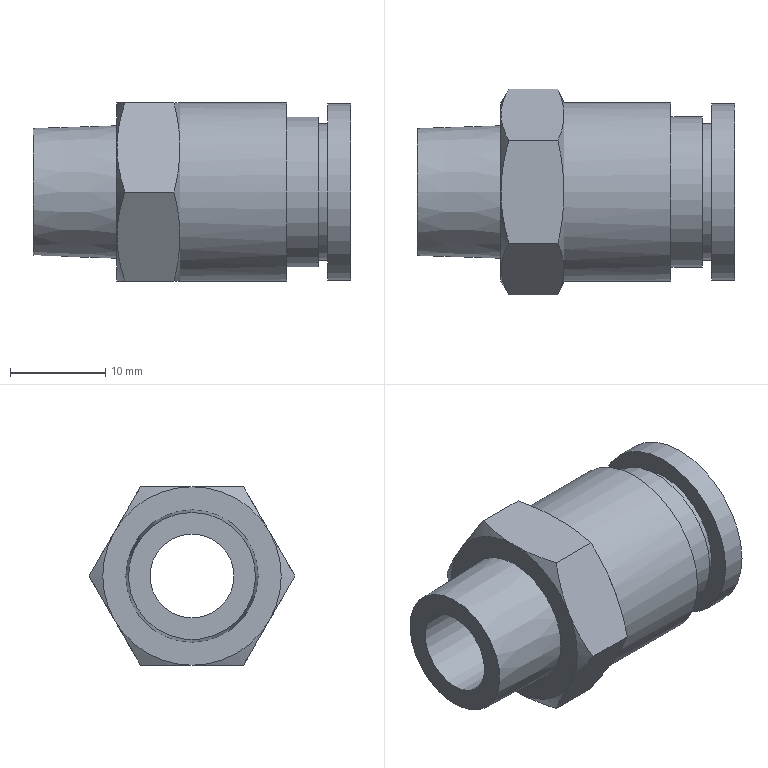Part | NX | features 模具.stp<1>[85] 2 | 1 solid | 32 faces | box 33.33 x 21.593 x 18.7 mm | volume 4989 mm3 | plane 13 | cone 13 | cylinder 6 | commonest cylinder face diameters 8.8 x1 11 x1 14.3 x1 15.73 x1 18.48 x1 18.7 x1
STEP:
#1=CARTESIAN_POINT('',(281.76,-25.,-59.9));
#2=VERTEX_POINT('',#1);
#3=CARTESIAN_POINT('',(281.76,-25.,-55.5));
#4=DIRECTION('',(-1.,0.,0.));
#5=DIRECTION('',(0.,0.,-1.));
#6=AXIS2_PLACEMENT_3D('',#3,#4,#5);
#7=CIRCLE('',#6,4.4);
#8=EDGE_CURVE('',#2,#2,#7,.T.);
#9=ORIENTED_EDGE('',*,*,#8,.F.);
#10=EDGE_LOOP('',(#9));
#11=FACE_BOUND('',#10,.T.);
#12=CARTESIAN_POINT('',(271.2,-25.,-51.1));
#13=VERTEX_POINT('',#12);
#14=CARTESIAN_POINT('',(271.2,-25.,-55.5));
#15=DIRECTION('',(-1.,0.,0.));
#16=DIRECTION('',(0.,0.,1.));
#17=AXIS2_PLACEMENT_3D('',#14,#15,#16);
#18=CIRCLE('',#17,4.4);
#19=EDGE_CURVE('',#13,#13,#18,.T.);
#20=ORIENTED_EDGE('',*,*,#19,.T.);
#21=EDGE_LOOP('',(#20));
#22=FACE_BOUND('',#21,.T.);
#23=CARTESIAN_POINT('',(304.53,-25.,-55.5));
#24=DIRECTION('',(1.,0.,0.));
#25=DIRECTION('',(0.,0.,1.));
#26=AXIS2_PLACEMENT_3D('',#23,#24,#25);
#27=CYLINDRICAL_SURFACE('',#26,4.4);
#28=ADVANCED_FACE('',(#11,#22),#27,.F.);
#29=ORIENTED_EDGE('',*,*,#8,.T.);
#30=EDGE_LOOP('',(#29));
#31=FACE_BOUND('',#30,.T.);
#32=CARTESIAN_POINT('',(281.76,-25.,-50.));
#33=VERTEX_POINT('',#32);
#34=CARTESIAN_POINT('',(281.76,-25.,-55.5));
#35=DIRECTION('',(-1.,0.,0.));
#36=DIRECTION('',(0.,0.,1.));
#37=AXIS2_PLACEMENT_3D('',#34,#35,#36);
#38=CIRCLE('',#37,5.5);
#39=EDGE_CURVE('',#33,#33,#38,.T.);
#40=ORIENTED_EDGE('',*,*,#39,.F.);
#41=EDGE_LOOP('',(#40));
#42=FACE_BOUND('',#41,.T.);
#43=CARTESIAN_POINT('',(281.76,-18.4,-48.9));
#44=DIRECTION('',(-1.,0.,0.));
#45=DIRECTION('',(0.,0.,1.));
#46=AXIS2_PLACEMENT_3D('',#43,#44,#45);
#47=PLANE('',#46);
#48=ADVANCED_FACE('',(#31,#42),#47,.F.);
#49=CARTESIAN_POINT('',(304.53,-25.,-61.));
#50=VERTEX_POINT('',#49);
#51=CARTESIAN_POINT('',(304.53,-25.,-55.5));
#52=DIRECTION('',(-1.,0.,0.));
#53=DIRECTION('',(0.,0.,-1.));
#54=AXIS2_PLACEMENT_3D('',#51,#52,#53);
#55=CIRCLE('',#54,5.5);
#56=EDGE_CURVE('',#50,#50,#55,.T.);
#57=ORIENTED_EDGE('',*,*,#56,.F.);
#58=EDGE_LOOP('',(#57));
#59=FACE_BOUND('',#58,.T.);
#60=ORIENTED_EDGE('',*,*,#39,.T.);
#61=EDGE_LOOP('',(#60));
#62=FACE_BOUND('',#61,.T.);
#63=CARTESIAN_POINT('',(304.53,-25.,-55.5));
#64=DIRECTION('',(1.,0.,0.));
#65=DIRECTION('',(0.,0.,1.));
#66=AXIS2_PLACEMENT_3D('',#63,#64,#65);
#67=CYLINDRICAL_SURFACE('',#66,5.5);
#68=ADVANCED_FACE('',(#59,#62),#67,.F.);
#69=ORIENTED_EDGE('',*,*,#56,.T.);
#70=EDGE_LOOP('',(#69));
#71=FACE_BOUND('',#70,.T.);
#72=CARTESIAN_POINT('',(304.53,-34.24,-55.5));
#73=VERTEX_POINT('',#72);
#74=CARTESIAN_POINT('',(304.53,-25.,-55.5));
#75=DIRECTION('',(1.,0.,0.));
#76=DIRECTION('',(0.,-1.,0.));
#77=AXIS2_PLACEMENT_3D('',#74,#75,#76);
#78=CIRCLE('',#77,9.24);
#79=EDGE_CURVE('',#73,#73,#78,.T.);
#80=ORIENTED_EDGE('',*,*,#79,.T.);
#81=EDGE_LOOP('',(#80));
#82=FACE_BOUND('',#81,.T.);
#83=CARTESIAN_POINT('',(304.53,-36.088,-66.588));
#84=DIRECTION('',(1.,0.,0.));
#85=DIRECTION('',(0.,1.,0.));
#86=AXIS2_PLACEMENT_3D('',#83,#84,#85);
#87=PLANE('',#86);
#88=ADVANCED_FACE('',(#71,#82),#87,.T.);
#89=CARTESIAN_POINT('',(302.11,-15.76,-55.5));
#90=VERTEX_POINT('',#89);
#91=CARTESIAN_POINT('',(302.11,-25.,-55.5));
#92=DIRECTION('',(1.,0.,0.));
#93=DIRECTION('',(0.,1.,0.));
#94=AXIS2_PLACEMENT_3D('',#91,#92,#93);
#95=CIRCLE('',#94,9.24);
#96=EDGE_CURVE('',#90,#90,#95,.T.);
#97=ORIENTED_EDGE('',*,*,#96,.T.);
#98=EDGE_LOOP('',(#97));
#99=FACE_BOUND('',#98,.T.);
#100=ORIENTED_EDGE('',*,*,#79,.F.);
#101=EDGE_LOOP('',(#100));
#102=FACE_BOUND('',#101,.T.);
#103=CARTESIAN_POINT('',(302.11,-25.,-55.5));
#104=DIRECTION('',(-1.,0.,0.));
#105=DIRECTION('',(0.,-1.,0.));
#106=AXIS2_PLACEMENT_3D('',#103,#104,#105);
#107=CYLINDRICAL_SURFACE('',#106,9.24);
#108=ADVANCED_FACE('',(#99,#102),#107,.T.);
#109=CARTESIAN_POINT('',(302.11,-32.15,-55.5));
#110=VERTEX_POINT('',#109);
#111=CARTESIAN_POINT('',(302.11,-25.,-55.5));
#112=DIRECTION('',(1.,0.,0.));
#113=DIRECTION('',(0.,-1.,0.));
#114=AXIS2_PLACEMENT_3D('',#111,#112,#113);
#115=CIRCLE('',#114,7.15);
#116=EDGE_CURVE('',#110,#110,#115,.T.);
#117=ORIENTED_EDGE('',*,*,#116,.T.);
#118=EDGE_LOOP('',(#117));
#119=FACE_BOUND('',#118,.T.);
#120=ORIENTED_EDGE('',*,*,#96,.F.);
#121=EDGE_LOOP('',(#120));
#122=FACE_BOUND('',#121,.T.);
#123=CARTESIAN_POINT('',(302.11,-36.088,-66.588));
#124=DIRECTION('',(1.,0.,0.));
#125=DIRECTION('',(0.,1.,0.));
#126=AXIS2_PLACEMENT_3D('',#123,#124,#125);
#127=PLANE('',#126);
#128=ADVANCED_FACE('',(#119,#122),#127,.F.);
#129=CARTESIAN_POINT('',(301.12,-17.85,-55.5));
#130=VERTEX_POINT('',#129);
#131=CARTESIAN_POINT('',(301.12,-25.,-55.5));
#132=DIRECTION('',(1.,0.,0.));
#133=DIRECTION('',(0.,1.,0.));
#134=AXIS2_PLACEMENT_3D('',#131,#132,#133);
#135=CIRCLE('',#134,7.15);
#136=EDGE_CURVE('',#130,#130,#135,.T.);
#137=ORIENTED_EDGE('',*,*,#136,.T.);
#138=EDGE_LOOP('',(#137));
#139=FACE_BOUND('',#138,.T.);
#140=ORIENTED_EDGE('',*,*,#116,.F.);
#141=EDGE_LOOP('',(#140));
#142=FACE_BOUND('',#141,.T.);
#143=CARTESIAN_POINT('',(301.12,-25.,-55.5));
#144=DIRECTION('',(-1.,0.,0.));
#145=DIRECTION('',(0.,-1.,0.));
#146=AXIS2_PLACEMENT_3D('',#143,#144,#145);
#147=CYLINDRICAL_SURFACE('',#146,7.15);
#148=ADVANCED_FACE('',(#139,#142),#147,.T.);
#149=ORIENTED_EDGE('',*,*,#136,.F.);
#150=EDGE_LOOP('',(#149));
#151=FACE_BOUND('',#150,.T.);
#152=CARTESIAN_POINT('',(301.12,-32.865,-55.5));
#153=VERTEX_POINT('',#152);
#154=CARTESIAN_POINT('',(301.12,-25.,-55.5));
#155=DIRECTION('',(1.,0.,0.));
#156=DIRECTION('',(0.,-1.,0.));
#157=AXIS2_PLACEMENT_3D('',#154,#155,#156);
#158=CIRCLE('',#157,7.865);
#159=EDGE_CURVE('',#153,#153,#158,.T.);
#160=ORIENTED_EDGE('',*,*,#159,.T.);
#161=EDGE_LOOP('',(#160));
#162=FACE_BOUND('',#161,.T.);
#163=CARTESIAN_POINT('',(301.12,-34.438,-64.938));
#164=DIRECTION('',(1.,0.,0.));
#165=DIRECTION('',(0.,1.,0.));
#166=AXIS2_PLACEMENT_3D('',#163,#164,#165);
#167=PLANE('',#166);
#168=ADVANCED_FACE('',(#151,#162),#167,.T.);
#169=CARTESIAN_POINT('',(297.82,-17.135,-55.5));
#170=VERTEX_POINT('',#169);
#171=CARTESIAN_POINT('',(297.82,-25.,-55.5));
#172=DIRECTION('',(1.,0.,0.));
#173=DIRECTION('',(0.,1.,0.));
#174=AXIS2_PLACEMENT_3D('',#171,#172,#173);
#175=CIRCLE('',#174,7.865);
#176=EDGE_CURVE('',#170,#170,#175,.T.);
#177=ORIENTED_EDGE('',*,*,#176,.T.);
#178=EDGE_LOOP('',(#177));
#179=FACE_BOUND('',#178,.T.);
#180=ORIENTED_EDGE('',*,*,#159,.F.);
#181=EDGE_LOOP('',(#180));
#182=FACE_BOUND('',#181,.T.);
#183=CARTESIAN_POINT('',(297.82,-25.,-55.5));
#184=DIRECTION('',(-1.,0.,0.));
#185=DIRECTION('',(0.,-1.,0.));
#186=AXIS2_PLACEMENT_3D('',#183,#184,#185);
#187=CYLINDRICAL_SURFACE('',#186,7.865);
#188=ADVANCED_FACE('',(#179,#182),#187,.T.);
#189=ORIENTED_EDGE('',*,*,#176,.F.);
#190=EDGE_LOOP('',(#189));
#191=FACE_BOUND('',#190,.T.);
#192=CARTESIAN_POINT('',(297.82,-15.65,-55.5));
#193=VERTEX_POINT('',#192);
#194=CARTESIAN_POINT('',(297.82,-25.,-55.5));
#195=DIRECTION('',(1.,0.,0.));
#196=DIRECTION('',(0.,1.,0.));
#197=AXIS2_PLACEMENT_3D('',#194,#195,#196);
#198=CIRCLE('',#197,9.35);
#199=EDGE_CURVE('',#193,#193,#198,.T.);
#200=ORIENTED_EDGE('',*,*,#199,.T.);
#201=EDGE_LOOP('',(#200));
#202=FACE_BOUND('',#201,.T.);
#203=CARTESIAN_POINT('',(297.82,-36.22,-66.72));
#204=DIRECTION('',(1.,0.,0.));
#205=DIRECTION('',(0.,1.,0.));
#206=AXIS2_PLACEMENT_3D('',#203,#204,#205);
#207=PLANE('',#206);
#208=ADVANCED_FACE('',(#191,#202),#207,.T.);
#209=CARTESIAN_POINT('',(285.975,-19.602,-46.15));
#210=VERTEX_POINT('',#209);
#211=CARTESIAN_POINT('',(286.6,-25.,-46.15));
#212=VERTEX_POINT('',#211);
#213=CARTESIAN_POINT('',(286.6,-25.,-46.15));
#214=CARTESIAN_POINT('',(286.6,-24.126,-46.15));
#215=CARTESIAN_POINT('',(286.487,-22.321,-46.15));
#216=CARTESIAN_POINT('',(286.183,-20.564,-46.15));
#217=CARTESIAN_POINT('',(285.975,-19.602,-46.15));
#218=B_SPLINE_CURVE_WITH_KNOTS('',3,(#213,#214,#215,#216,#217),.UNSPECIFIED.,.F.,.F.,(4,1,4),(0.,0.5,1.),.UNSPECIFIED.);
#219=EDGE_CURVE('',#210,#212,#218,.F.);
#220=ORIENTED_EDGE('',*,*,#219,.F.);
#221=CARTESIAN_POINT('',(280.835,-19.602,-46.15));
#222=VERTEX_POINT('',#221);
#223=CARTESIAN_POINT('',(280.835,-19.602,-46.15));
#224=DIRECTION('',(1.,0.,0.));
#225=VECTOR('',#224,1000.);
#226=LINE('',#223,#225);
#227=EDGE_CURVE('',#222,#210,#226,.T.);
#228=ORIENTED_EDGE('',*,*,#227,.F.);
#229=CARTESIAN_POINT('',(280.,-25.,-46.15));
#230=VERTEX_POINT('',#229);
#231=CARTESIAN_POINT('',(280.835,-19.602,-46.15));
#232=CARTESIAN_POINT('',(280.557,-20.566,-46.15));
#233=CARTESIAN_POINT('',(280.149,-22.33,-46.15));
#234=CARTESIAN_POINT('',(280.,-24.127,-46.15));
#235=CARTESIAN_POINT('',(280.,-25.,-46.15));
#236=B_SPLINE_CURVE_WITH_KNOTS('',3,(#231,#232,#233,#234,#235),.UNSPECIFIED.,.F.,.F.,(4,1,4),(0.,0.5,1.),.UNSPECIFIED.);
#237=EDGE_CURVE('',#230,#222,#236,.F.);
#238=ORIENTED_EDGE('',*,*,#237,.F.);
#239=CARTESIAN_POINT('',(280.835,-30.398,-46.15));
#240=VERTEX_POINT('',#239);
#241=CARTESIAN_POINT('',(280.,-25.,-46.15));
#242=CARTESIAN_POINT('',(280.,-25.871,-46.15));
#243=CARTESIAN_POINT('',(280.147,-27.657,-46.15));
#244=CARTESIAN_POINT('',(280.556,-29.43,-46.15));
#245=CARTESIAN_POINT('',(280.835,-30.398,-46.15));
#246=B_SPLINE_CURVE_WITH_KNOTS('',3,(#241,#242,#243,#244,#245),.UNSPECIFIED.,.F.,.F.,(4,1,4),(0.,0.5,1.),.UNSPECIFIED.);
#247=EDGE_CURVE('',#240,#230,#246,.F.);
#248=ORIENTED_EDGE('',*,*,#247,.F.);
#249=CARTESIAN_POINT('',(285.975,-30.398,-46.15));
#250=VERTEX_POINT('',#249);
#251=CARTESIAN_POINT('',(280.835,-30.398,-46.15));
#252=DIRECTION('',(1.,0.,0.));
#253=VECTOR('',#252,1000.);
#254=LINE('',#251,#253);
#255=EDGE_CURVE('',#240,#250,#254,.T.);
#256=ORIENTED_EDGE('',*,*,#255,.T.);
#257=CARTESIAN_POINT('',(285.975,-30.398,-46.15));
#258=CARTESIAN_POINT('',(286.182,-29.439,-46.15));
#259=CARTESIAN_POINT('',(286.486,-27.691,-46.15));
#260=CARTESIAN_POINT('',(286.6,-25.876,-46.15));
#261=CARTESIAN_POINT('',(286.6,-25.,-46.15));
#262=B_SPLINE_CURVE_WITH_KNOTS('',3,(#257,#258,#259,#260,#261),.UNSPECIFIED.,.F.,.F.,(4,1,4),(0.,0.5,1.),.UNSPECIFIED.);
#263=EDGE_CURVE('',#212,#250,#262,.F.);
#264=ORIENTED_EDGE('',*,*,#263,.F.);
#265=EDGE_LOOP('',(#220,#228,#238,#248,#256,#264));
#266=FACE_BOUND('',#265,.T.);
#267=CARTESIAN_POINT('',(287.26,-18.522,-46.15));
#268=DIRECTION('',(0.,0.,1.));
#269=DIRECTION('',(1.,0.,0.));
#270=AXIS2_PLACEMENT_3D('',#267,#268,#269);
#271=PLANE('',#270);
#272=ADVANCED_FACE('',(#266),#271,.T.);
#273=ORIENTED_EDGE('',*,*,#255,.F.);
#274=CARTESIAN_POINT('',(280.,-33.097,-50.825));
#275=VERTEX_POINT('',#274);
#276=CARTESIAN_POINT('',(280.835,-30.398,-46.15));
#277=CARTESIAN_POINT('',(280.275,-31.368,-47.831));
#278=CARTESIAN_POINT('',(280.,-32.228,-49.319));
#279=CARTESIAN_POINT('',(280.,-33.097,-50.825));
#280=B_SPLINE_CURVE_WITH_KNOTS('',3,(#276,#277,#278,#279),.UNSPECIFIED.,.F.,.F.,(4,4),(0.,1.),.UNSPECIFIED.);
#281=EDGE_CURVE('',#275,#240,#280,.F.);
#282=ORIENTED_EDGE('',*,*,#281,.F.);
#283=CARTESIAN_POINT('',(280.835,-35.796,-55.5));
#284=VERTEX_POINT('',#283);
#285=CARTESIAN_POINT('',(280.,-33.097,-50.825));
#286=CARTESIAN_POINT('',(280.,-33.966,-52.33));
#287=CARTESIAN_POINT('',(280.275,-34.826,-53.819));
#288=CARTESIAN_POINT('',(280.835,-35.796,-55.5));
#289=B_SPLINE_CURVE_WITH_KNOTS('',3,(#285,#286,#287,#288),.UNSPECIFIED.,.F.,.F.,(4,4),(0.,1.),.UNSPECIFIED.);
#290=EDGE_CURVE('',#284,#275,#289,.F.);
#291=ORIENTED_EDGE('',*,*,#290,.F.);
#292=CARTESIAN_POINT('',(285.975,-35.796,-55.5));
#293=VERTEX_POINT('',#292);
#294=CARTESIAN_POINT('',(280.835,-35.796,-55.5));
#295=DIRECTION('',(1.,0.,0.));
#296=VECTOR('',#295,1000.);
#297=LINE('',#294,#296);
#298=EDGE_CURVE('',#284,#293,#297,.T.);
#299=ORIENTED_EDGE('',*,*,#298,.T.);
#300=CARTESIAN_POINT('',(286.6,-33.097,-50.825));
#301=VERTEX_POINT('',#300);
#302=CARTESIAN_POINT('',(285.975,-35.796,-55.5));
#303=CARTESIAN_POINT('',(286.183,-35.314,-54.665));
#304=CARTESIAN_POINT('',(286.489,-34.431,-53.136));
#305=CARTESIAN_POINT('',(286.6,-33.534,-51.581));
#306=CARTESIAN_POINT('',(286.6,-33.097,-50.825));
#307=B_SPLINE_CURVE_WITH_KNOTS('',3,(#302,#303,#304,#305,#306),.UNSPECIFIED.,.F.,.F.,(4,1,4),(0.,0.5,1.),.UNSPECIFIED.);
#308=EDGE_CURVE('',#301,#293,#307,.F.);
#309=ORIENTED_EDGE('',*,*,#308,.F.);
#310=CARTESIAN_POINT('',(286.6,-33.097,-50.825));
#311=CARTESIAN_POINT('',(286.6,-32.661,-50.069));
#312=CARTESIAN_POINT('',(286.489,-31.763,-48.514));
#313=CARTESIAN_POINT('',(286.184,-30.881,-46.986));
#314=CARTESIAN_POINT('',(285.975,-30.398,-46.15));
#315=B_SPLINE_CURVE_WITH_KNOTS('',3,(#310,#311,#312,#313,#314),.UNSPECIFIED.,.F.,.F.,(4,1,4),(0.,0.5,1.),.UNSPECIFIED.);
#316=EDGE_CURVE('',#250,#301,#315,.F.);
#317=ORIENTED_EDGE('',*,*,#316,.F.);
#318=EDGE_LOOP('',(#273,#282,#291,#299,#309,#317));
#319=FACE_BOUND('',#318,.T.);
#320=CARTESIAN_POINT('',(287.26,-29.858,-45.215));
#321=DIRECTION('',(0.,-0.866,0.5));
#322=DIRECTION('',(-1.,0.,0.));
#323=AXIS2_PLACEMENT_3D('',#320,#321,#322);
#324=PLANE('',#323);
#325=ADVANCED_FACE('',(#319),#324,.T.);
#326=CARTESIAN_POINT('',(280.,-25.,-55.5));
#327=DIRECTION('',(-1.,0.,0.));
#328=DIRECTION('',(0.,0.866,-0.5));
#329=AXIS2_PLACEMENT_3D('',#326,#327,#328);
#330=CIRCLE('',#329,9.35);
#331=EDGE_CURVE('',#275,#230,#330,.T.);
#332=ORIENTED_EDGE('',*,*,#331,.F.);
#333=ORIENTED_EDGE('',*,*,#281,.T.);
#334=ORIENTED_EDGE('',*,*,#247,.T.);
#335=EDGE_LOOP('',(#332,#333,#334));
#336=FACE_BOUND('',#335,.T.);
#337=CARTESIAN_POINT('',(281.744,-25.,-55.5));
#338=DIRECTION('',(1.,0.,0.));
#339=DIRECTION('',(0.,-0.8661,0.4999));
#340=AXIS2_PLACEMENT_3D('',#337,#338,#339);
#341=CONICAL_SURFACE('',#340,12.37,1.047);
#342=ADVANCED_FACE('',(#336),#341,.T.);
#343=CARTESIAN_POINT('',(280.,-33.097,-60.175));
#344=VERTEX_POINT('',#343);
#345=CARTESIAN_POINT('',(280.,-25.,-55.5));
#346=DIRECTION('',(-1.,0.,0.));
#347=DIRECTION('',(0.,0.866,0.5));
#348=AXIS2_PLACEMENT_3D('',#345,#346,#347);
#349=CIRCLE('',#348,9.35);
#350=EDGE_CURVE('',#344,#275,#349,.T.);
#351=ORIENTED_EDGE('',*,*,#350,.F.);
#352=CARTESIAN_POINT('',(280.835,-35.796,-55.5));
#353=CARTESIAN_POINT('',(280.275,-34.826,-57.181));
#354=CARTESIAN_POINT('',(280.,-33.967,-58.669));
#355=CARTESIAN_POINT('',(280.,-33.097,-60.175));
#356=B_SPLINE_CURVE_WITH_KNOTS('',3,(#352,#353,#354,#355),.UNSPECIFIED.,.F.,.F.,(4,4),(0.,1.),.UNSPECIFIED.);
#357=EDGE_CURVE('',#344,#284,#356,.F.);
#358=ORIENTED_EDGE('',*,*,#357,.T.);
#359=ORIENTED_EDGE('',*,*,#290,.T.);
#360=EDGE_LOOP('',(#351,#358,#359));
#361=FACE_BOUND('',#360,.T.);
#362=CARTESIAN_POINT('',(281.395,-25.,-55.5));
#363=DIRECTION('',(1.,0.,0.));
#364=DIRECTION('',(0.,0.,1.));
#365=AXIS2_PLACEMENT_3D('',#362,#363,#364);
#366=CONICAL_SURFACE('',#365,11.767,1.047);
#367=ADVANCED_FACE('',(#361),#366,.T.);
#368=CARTESIAN_POINT('',(280.,-25.,-64.85));
#369=VERTEX_POINT('',#368);
#370=CARTESIAN_POINT('',(280.,-25.,-55.5));
#371=DIRECTION('',(-1.,0.,0.));
#372=DIRECTION('',(0.,0.,1.));
#373=AXIS2_PLACEMENT_3D('',#370,#371,#372);
#374=CIRCLE('',#373,9.35);
#375=EDGE_CURVE('',#369,#344,#374,.T.);
#376=ORIENTED_EDGE('',*,*,#375,.F.);
#377=CARTESIAN_POINT('',(280.835,-30.398,-64.85));
#378=VERTEX_POINT('',#377);
#379=CARTESIAN_POINT('',(280.835,-30.398,-64.85));
#380=CARTESIAN_POINT('',(280.557,-29.434,-64.85));
#381=CARTESIAN_POINT('',(280.149,-27.67,-64.85));
#382=CARTESIAN_POINT('',(280.,-25.873,-64.85));
#383=CARTESIAN_POINT('',(280.,-25.,-64.85));
#384=B_SPLINE_CURVE_WITH_KNOTS('',3,(#379,#380,#381,#382,#383),.UNSPECIFIED.,.F.,.F.,(4,1,4),(0.,0.5,1.),.UNSPECIFIED.);
#385=EDGE_CURVE('',#369,#378,#384,.F.);
#386=ORIENTED_EDGE('',*,*,#385,.T.);
#387=CARTESIAN_POINT('',(280.,-33.097,-60.175));
#388=CARTESIAN_POINT('',(280.,-32.228,-61.68));
#389=CARTESIAN_POINT('',(280.275,-31.369,-63.169));
#390=CARTESIAN_POINT('',(280.835,-30.398,-64.85));
#391=B_SPLINE_CURVE_WITH_KNOTS('',3,(#387,#388,#389,#390),.UNSPECIFIED.,.F.,.F.,(4,4),(0.,1.),.UNSPECIFIED.);
#392=EDGE_CURVE('',#378,#344,#391,.F.);
#393=ORIENTED_EDGE('',*,*,#392,.T.);
#394=EDGE_LOOP('',(#376,#386,#393));
#395=FACE_BOUND('',#394,.T.);
#396=CARTESIAN_POINT('',(281.744,-25.,-55.5));
#397=DIRECTION('',(1.,0.,0.));
#398=DIRECTION('',(0.,0.,1.));
#399=AXIS2_PLACEMENT_3D('',#396,#397,#398);
#400=CONICAL_SURFACE('',#399,12.37,1.047);
#401=ADVANCED_FACE('',(#395),#400,.T.);
#402=CARTESIAN_POINT('',(280.835,-19.602,-64.85));
#403=VERTEX_POINT('',#402);
#404=CARTESIAN_POINT('',(285.975,-19.602,-64.85));
#405=VERTEX_POINT('',#404);
#406=CARTESIAN_POINT('',(280.835,-19.602,-64.85));
#407=DIRECTION('',(1.,0.,0.));
#408=VECTOR('',#407,1000.);
#409=LINE('',#406,#408);
#410=EDGE_CURVE('',#403,#405,#409,.T.);
#411=ORIENTED_EDGE('',*,*,#410,.F.);
#412=CARTESIAN_POINT('',(280.,-16.903,-60.175));
#413=VERTEX_POINT('',#412);
#414=CARTESIAN_POINT('',(280.835,-19.602,-64.85));
#415=CARTESIAN_POINT('',(280.275,-18.632,-63.169));
#416=CARTESIAN_POINT('',(280.,-17.772,-61.681));
#417=CARTESIAN_POINT('',(280.,-16.903,-60.175));
#418=B_SPLINE_CURVE_WITH_KNOTS('',3,(#414,#415,#416,#417),.UNSPECIFIED.,.F.,.F.,(4,4),(0.,1.),.UNSPECIFIED.);
#419=EDGE_CURVE('',#413,#403,#418,.F.);
#420=ORIENTED_EDGE('',*,*,#419,.F.);
#421=CARTESIAN_POINT('',(280.835,-14.204,-55.5));
#422=VERTEX_POINT('',#421);
#423=CARTESIAN_POINT('',(280.,-16.903,-60.175));
#424=CARTESIAN_POINT('',(280.,-16.034,-58.67));
#425=CARTESIAN_POINT('',(280.275,-15.174,-57.181));
#426=CARTESIAN_POINT('',(280.835,-14.204,-55.5));
#427=B_SPLINE_CURVE_WITH_KNOTS('',3,(#423,#424,#425,#426),.UNSPECIFIED.,.F.,.F.,(4,4),(0.,1.),.UNSPECIFIED.);
#428=EDGE_CURVE('',#422,#413,#427,.F.);
#429=ORIENTED_EDGE('',*,*,#428,.F.);
#430=CARTESIAN_POINT('',(285.975,-14.204,-55.5));
#431=VERTEX_POINT('',#430);
#432=CARTESIAN_POINT('',(280.835,-14.204,-55.5));
#433=DIRECTION('',(1.,0.,0.));
#434=VECTOR('',#433,1000.);
#435=LINE('',#432,#434);
#436=EDGE_CURVE('',#422,#431,#435,.T.);
#437=ORIENTED_EDGE('',*,*,#436,.T.);
#438=CARTESIAN_POINT('',(286.6,-16.903,-60.175));
#439=VERTEX_POINT('',#438);
#440=CARTESIAN_POINT('',(285.975,-14.204,-55.5));
#441=CARTESIAN_POINT('',(286.183,-14.686,-56.335));
#442=CARTESIAN_POINT('',(286.489,-15.569,-57.864));
#443=CARTESIAN_POINT('',(286.6,-16.466,-59.419));
#444=CARTESIAN_POINT('',(286.6,-16.903,-60.175));
#445=B_SPLINE_CURVE_WITH_KNOTS('',3,(#440,#441,#442,#443,#444),.UNSPECIFIED.,.F.,.F.,(4,1,4),(0.,0.5,1.),.UNSPECIFIED.);
#446=EDGE_CURVE('',#439,#431,#445,.F.);
#447=ORIENTED_EDGE('',*,*,#446,.F.);
#448=CARTESIAN_POINT('',(286.6,-16.903,-60.175));
#449=CARTESIAN_POINT('',(286.6,-17.339,-60.931));
#450=CARTESIAN_POINT('',(286.489,-18.237,-62.486));
#451=CARTESIAN_POINT('',(286.184,-19.119,-64.014));
#452=CARTESIAN_POINT('',(285.975,-19.602,-64.85));
#453=B_SPLINE_CURVE_WITH_KNOTS('',3,(#448,#449,#450,#451,#452),.UNSPECIFIED.,.F.,.F.,(4,1,4),(0.,0.5,1.),.UNSPECIFIED.);
#454=EDGE_CURVE('',#405,#439,#453,.F.);
#455=ORIENTED_EDGE('',*,*,#454,.F.);
#456=EDGE_LOOP('',(#411,#420,#429,#437,#447,#455));
#457=FACE_BOUND('',#456,.T.);
#458=CARTESIAN_POINT('',(279.34,-13.664,-54.565));
#459=DIRECTION('',(0.,0.866,-0.5));
#460=DIRECTION('',(-1.,0.,0.));
#461=AXIS2_PLACEMENT_3D('',#458,#459,#460);
#462=PLANE('',#461);
#463=ADVANCED_FACE('',(#457),#462,.T.);
#464=CARTESIAN_POINT('',(285.975,-30.398,-64.85));
#465=VERTEX_POINT('',#464);
#466=CARTESIAN_POINT('',(280.835,-30.398,-64.85));
#467=DIRECTION('',(1.,0.,0.));
#468=VECTOR('',#467,1000.);
#469=LINE('',#466,#468);
#470=EDGE_CURVE('',#378,#465,#469,.T.);
#471=ORIENTED_EDGE('',*,*,#470,.F.);
#472=ORIENTED_EDGE('',*,*,#385,.F.);
#473=CARTESIAN_POINT('',(280.,-25.,-64.85));
#474=CARTESIAN_POINT('',(280.,-24.129,-64.85));
#475=CARTESIAN_POINT('',(280.147,-22.343,-64.85));
#476=CARTESIAN_POINT('',(280.556,-20.57,-64.85));
#477=CARTESIAN_POINT('',(280.835,-19.602,-64.85));
#478=B_SPLINE_CURVE_WITH_KNOTS('',3,(#473,#474,#475,#476,#477),.UNSPECIFIED.,.F.,.F.,(4,1,4),(0.,0.5,1.),.UNSPECIFIED.);
#479=EDGE_CURVE('',#403,#369,#478,.F.);
#480=ORIENTED_EDGE('',*,*,#479,.F.);
#481=ORIENTED_EDGE('',*,*,#410,.T.);
#482=CARTESIAN_POINT('',(286.6,-25.,-64.85));
#483=VERTEX_POINT('',#482);
#484=CARTESIAN_POINT('',(285.975,-19.602,-64.85));
#485=CARTESIAN_POINT('',(286.182,-20.561,-64.85));
#486=CARTESIAN_POINT('',(286.486,-22.309,-64.85));
#487=CARTESIAN_POINT('',(286.6,-24.124,-64.85));
#488=CARTESIAN_POINT('',(286.6,-25.,-64.85));
#489=B_SPLINE_CURVE_WITH_KNOTS('',3,(#484,#485,#486,#487,#488),.UNSPECIFIED.,.F.,.F.,(4,1,4),(0.,0.5,1.),.UNSPECIFIED.);
#490=EDGE_CURVE('',#483,#405,#489,.F.);
#491=ORIENTED_EDGE('',*,*,#490,.F.);
#492=CARTESIAN_POINT('',(286.6,-25.,-64.85));
#493=CARTESIAN_POINT('',(286.6,-25.874,-64.85));
#494=CARTESIAN_POINT('',(286.487,-27.679,-64.85));
#495=CARTESIAN_POINT('',(286.183,-29.436,-64.85));
#496=CARTESIAN_POINT('',(285.975,-30.398,-64.85));
#497=B_SPLINE_CURVE_WITH_KNOTS('',3,(#492,#493,#494,#495,#496),.UNSPECIFIED.,.F.,.F.,(4,1,4),(0.,0.5,1.),.UNSPECIFIED.);
#498=EDGE_CURVE('',#465,#483,#497,.F.);
#499=ORIENTED_EDGE('',*,*,#498,.F.);
#500=EDGE_LOOP('',(#471,#472,#480,#481,#491,#499));
#501=FACE_BOUND('',#500,.T.);
#502=CARTESIAN_POINT('',(287.26,-18.522,-64.85));
#503=DIRECTION('',(0.,0.,-1.));
#504=DIRECTION('',(0.,-1.,0.));
#505=AXIS2_PLACEMENT_3D('',#502,#503,#504);
#506=PLANE('',#505);
#507=ADVANCED_FACE('',(#501),#506,.T.);
#508=ORIENTED_EDGE('',*,*,#298,.F.);
#509=ORIENTED_EDGE('',*,*,#357,.F.);
#510=ORIENTED_EDGE('',*,*,#392,.F.);
#511=ORIENTED_EDGE('',*,*,#470,.T.);
#512=CARTESIAN_POINT('',(286.6,-33.097,-60.175));
#513=VERTEX_POINT('',#512);
#514=CARTESIAN_POINT('',(285.975,-30.398,-64.85));
#515=CARTESIAN_POINT('',(286.183,-30.881,-64.015));
#516=CARTESIAN_POINT('',(286.489,-31.763,-62.486));
#517=CARTESIAN_POINT('',(286.6,-32.661,-60.931));
#518=CARTESIAN_POINT('',(286.6,-33.097,-60.175));
#519=B_SPLINE_CURVE_WITH_KNOTS('',3,(#514,#515,#516,#517,#518),.UNSPECIFIED.,.F.,.F.,(4,1,4),(0.,0.5,1.),.UNSPECIFIED.);
#520=EDGE_CURVE('',#513,#465,#519,.F.);
#521=ORIENTED_EDGE('',*,*,#520,.F.);
#522=CARTESIAN_POINT('',(286.6,-33.097,-60.175));
#523=CARTESIAN_POINT('',(286.6,-33.534,-59.419));
#524=CARTESIAN_POINT('',(286.489,-34.432,-57.864));
#525=CARTESIAN_POINT('',(286.184,-35.314,-56.336));
#526=CARTESIAN_POINT('',(285.975,-35.796,-55.5));
#527=B_SPLINE_CURVE_WITH_KNOTS('',3,(#522,#523,#524,#525,#526),.UNSPECIFIED.,.F.,.F.,(4,1,4),(0.,0.5,1.),.UNSPECIFIED.);
#528=EDGE_CURVE('',#293,#513,#527,.F.);
#529=ORIENTED_EDGE('',*,*,#528,.F.);
#530=EDGE_LOOP('',(#508,#509,#510,#511,#521,#529));
#531=FACE_BOUND('',#530,.T.);
#532=CARTESIAN_POINT('',(279.34,-29.858,-65.785));
#533=DIRECTION('',(0.,-0.866,-0.5));
#534=DIRECTION('',(0.,0.5,-0.866));
#535=AXIS2_PLACEMENT_3D('',#532,#533,#534);
#536=PLANE('',#535);
#537=ADVANCED_FACE('',(#531),#536,.T.);
#538=ORIENTED_EDGE('',*,*,#263,.T.);
#539=ORIENTED_EDGE('',*,*,#316,.T.);
#540=CARTESIAN_POINT('',(286.6,-25.,-55.5));
#541=DIRECTION('',(1.,0.,0.));
#542=DIRECTION('',(0.,0.,-1.));
#543=AXIS2_PLACEMENT_3D('',#540,#541,#542);
#544=CIRCLE('',#543,9.35);
#545=EDGE_CURVE('',#212,#301,#544,.T.);
#546=ORIENTED_EDGE('',*,*,#545,.F.);
#547=EDGE_LOOP('',(#538,#539,#546));
#548=FACE_BOUND('',#547,.T.);
#549=CARTESIAN_POINT('',(285.295,-25.,-55.5));
#550=DIRECTION('',(-1.,0.,0.));
#551=DIRECTION('',(0.,0.,-1.));
#552=AXIS2_PLACEMENT_3D('',#549,#550,#551);
#553=CONICAL_SURFACE('',#552,12.37,1.163);
#554=ADVANCED_FACE('',(#548),#553,.T.);
#555=ORIENTED_EDGE('',*,*,#520,.T.);
#556=ORIENTED_EDGE('',*,*,#498,.T.);
#557=CARTESIAN_POINT('',(286.6,-25.,-55.5));
#558=DIRECTION('',(1.,0.,0.));
#559=DIRECTION('',(0.,0.866,0.5));
#560=AXIS2_PLACEMENT_3D('',#557,#558,#559);
#561=CIRCLE('',#560,9.35);
#562=EDGE_CURVE('',#513,#483,#561,.T.);
#563=ORIENTED_EDGE('',*,*,#562,.F.);
#564=EDGE_LOOP('',(#555,#556,#563));
#565=FACE_BOUND('',#564,.T.);
#566=CARTESIAN_POINT('',(285.295,-25.,-55.5));
#567=DIRECTION('',(-1.,0.,0.));
#568=DIRECTION('',(0.,-0.8661,-0.4999));
#569=AXIS2_PLACEMENT_3D('',#566,#567,#568);
#570=CONICAL_SURFACE('',#569,12.37,1.163);
#571=ADVANCED_FACE('',(#565),#570,.T.);
#572=CARTESIAN_POINT('',(286.6,-25.,-55.5));
#573=DIRECTION('',(1.,0.,0.));
#574=DIRECTION('',(0.,1.,0.));
#575=AXIS2_PLACEMENT_3D('',#572,#573,#574);
#576=CIRCLE('',#575,9.35);
#577=EDGE_CURVE('',#301,#513,#576,.T.);
#578=ORIENTED_EDGE('',*,*,#577,.F.);
#579=ORIENTED_EDGE('',*,*,#308,.T.);
#580=ORIENTED_EDGE('',*,*,#528,.T.);
#581=EDGE_LOOP('',(#578,#579,#580));
#582=FACE_BOUND('',#581,.T.);
#583=CARTESIAN_POINT('',(285.556,-25.,-55.5));
#584=DIRECTION('',(-1.,0.,0.));
#585=DIRECTION('',(0.,0.,-1.));
#586=AXIS2_PLACEMENT_3D('',#583,#584,#585);
#587=CONICAL_SURFACE('',#586,11.767,1.163);
#588=ADVANCED_FACE('',(#582),#587,.T.);
#589=ORIENTED_EDGE('',*,*,#562,.T.);
#590=CARTESIAN_POINT('',(286.6,-25.,-55.5));
#591=DIRECTION('',(1.,0.,0.));
#592=DIRECTION('',(0.,0.,1.));
#593=AXIS2_PLACEMENT_3D('',#590,#591,#592);
#594=CIRCLE('',#593,9.35);
#595=EDGE_CURVE('',#483,#439,#594,.T.);
#596=ORIENTED_EDGE('',*,*,#595,.T.);
#597=CARTESIAN_POINT('',(286.6,-16.903,-50.825));
#598=VERTEX_POINT('',#597);
#599=CARTESIAN_POINT('',(286.6,-25.,-55.5));
#600=DIRECTION('',(1.,0.,0.));
#601=DIRECTION('',(0.,-1.,0.));
#602=AXIS2_PLACEMENT_3D('',#599,#600,#601);
#603=CIRCLE('',#602,9.35);
#604=EDGE_CURVE('',#439,#598,#603,.T.);
#605=ORIENTED_EDGE('',*,*,#604,.T.);
#606=CARTESIAN_POINT('',(286.6,-25.,-55.5));
#607=DIRECTION('',(1.,0.,0.));
#608=DIRECTION('',(0.,-0.866,-0.5));
#609=AXIS2_PLACEMENT_3D('',#606,#607,#608);
#610=CIRCLE('',#609,9.35);
#611=EDGE_CURVE('',#598,#212,#610,.T.);
#612=ORIENTED_EDGE('',*,*,#611,.T.);
#613=ORIENTED_EDGE('',*,*,#545,.T.);
#614=ORIENTED_EDGE('',*,*,#577,.T.);
#615=EDGE_LOOP('',(#589,#596,#605,#612,#613,#614));
#616=FACE_BOUND('',#615,.T.);
#617=ORIENTED_EDGE('',*,*,#199,.F.);
#618=EDGE_LOOP('',(#617));
#619=FACE_BOUND('',#618,.T.);
#620=CARTESIAN_POINT('',(286.6,-25.,-55.5));
#621=DIRECTION('',(-1.,0.,0.));
#622=DIRECTION('',(0.,1.,0.));
#623=AXIS2_PLACEMENT_3D('',#620,#621,#622);
#624=CYLINDRICAL_SURFACE('',#623,9.35);
#625=ADVANCED_FACE('',(#616,#619),#624,.T.);
#626=CARTESIAN_POINT('',(285.975,-19.602,-46.15));
#627=CARTESIAN_POINT('',(286.183,-19.119,-46.985));
#628=CARTESIAN_POINT('',(286.489,-18.237,-48.514));
#629=CARTESIAN_POINT('',(286.6,-17.339,-50.069));
#630=CARTESIAN_POINT('',(286.6,-16.903,-50.825));
#631=B_SPLINE_CURVE_WITH_KNOTS('',3,(#626,#627,#628,#629,#630),.UNSPECIFIED.,.F.,.F.,(4,1,4),(0.,0.5,1.),.UNSPECIFIED.);
#632=EDGE_CURVE('',#598,#210,#631,.F.);
#633=ORIENTED_EDGE('',*,*,#632,.T.);
#634=ORIENTED_EDGE('',*,*,#219,.T.);
#635=ORIENTED_EDGE('',*,*,#611,.F.);
#636=EDGE_LOOP('',(#633,#634,#635));
#637=FACE_BOUND('',#636,.T.);
#638=CARTESIAN_POINT('',(285.295,-25.,-55.5));
#639=DIRECTION('',(-1.,0.,0.));
#640=DIRECTION('',(0.,0.,-1.));
#641=AXIS2_PLACEMENT_3D('',#638,#639,#640);
#642=CONICAL_SURFACE('',#641,12.37,1.163);
#643=ADVANCED_FACE('',(#637),#642,.T.);
#644=ORIENTED_EDGE('',*,*,#446,.T.);
#645=CARTESIAN_POINT('',(286.6,-16.903,-50.825));
#646=CARTESIAN_POINT('',(286.6,-16.466,-51.581));
#647=CARTESIAN_POINT('',(286.489,-15.568,-53.136));
#648=CARTESIAN_POINT('',(286.184,-14.686,-54.664));
#649=CARTESIAN_POINT('',(285.975,-14.204,-55.5));
#650=B_SPLINE_CURVE_WITH_KNOTS('',3,(#645,#646,#647,#648,#649),.UNSPECIFIED.,.F.,.F.,(4,1,4),(0.,0.5,1.),.UNSPECIFIED.);
#651=EDGE_CURVE('',#431,#598,#650,.F.);
#652=ORIENTED_EDGE('',*,*,#651,.T.);
#653=ORIENTED_EDGE('',*,*,#604,.F.);
#654=EDGE_LOOP('',(#644,#652,#653));
#655=FACE_BOUND('',#654,.T.);
#656=CARTESIAN_POINT('',(285.556,-25.,-55.5));
#657=DIRECTION('',(-1.,0.,0.));
#658=DIRECTION('',(0.,0.,-1.));
#659=AXIS2_PLACEMENT_3D('',#656,#657,#658);
#660=CONICAL_SURFACE('',#659,11.767,1.163);
#661=ADVANCED_FACE('',(#655),#660,.T.);
#662=ORIENTED_EDGE('',*,*,#490,.T.);
#663=ORIENTED_EDGE('',*,*,#454,.T.);
#664=ORIENTED_EDGE('',*,*,#595,.F.);
#665=EDGE_LOOP('',(#662,#663,#664));
#666=FACE_BOUND('',#665,.T.);
#667=CARTESIAN_POINT('',(285.295,-25.,-55.5));
#668=DIRECTION('',(-1.,0.,0.));
#669=DIRECTION('',(0.,-0.0002353,-1.));
#670=AXIS2_PLACEMENT_3D('',#667,#668,#669);
#671=CONICAL_SURFACE('',#670,12.37,1.163);
#672=ADVANCED_FACE('',(#666),#671,.T.);
#673=ORIENTED_EDGE('',*,*,#436,.F.);
#674=CARTESIAN_POINT('',(280.,-16.903,-50.825));
#675=VERTEX_POINT('',#674);
#676=CARTESIAN_POINT('',(280.835,-14.204,-55.5));
#677=CARTESIAN_POINT('',(280.275,-15.174,-53.819));
#678=CARTESIAN_POINT('',(280.,-16.033,-52.331));
#679=CARTESIAN_POINT('',(280.,-16.903,-50.825));
#680=B_SPLINE_CURVE_WITH_KNOTS('',3,(#676,#677,#678,#679),.UNSPECIFIED.,.F.,.F.,(4,4),(0.,1.),.UNSPECIFIED.);
#681=EDGE_CURVE('',#675,#422,#680,.F.);
#682=ORIENTED_EDGE('',*,*,#681,.F.);
#683=CARTESIAN_POINT('',(280.,-16.903,-50.825));
#684=CARTESIAN_POINT('',(280.,-17.772,-49.32));
#685=CARTESIAN_POINT('',(280.275,-18.631,-47.831));
#686=CARTESIAN_POINT('',(280.835,-19.602,-46.15));
#687=B_SPLINE_CURVE_WITH_KNOTS('',3,(#683,#684,#685,#686),.UNSPECIFIED.,.F.,.F.,(4,4),(0.,1.),.UNSPECIFIED.);
#688=EDGE_CURVE('',#222,#675,#687,.F.);
#689=ORIENTED_EDGE('',*,*,#688,.F.);
#690=ORIENTED_EDGE('',*,*,#227,.T.);
#691=ORIENTED_EDGE('',*,*,#632,.F.);
#692=ORIENTED_EDGE('',*,*,#651,.F.);
#693=EDGE_LOOP('',(#673,#682,#689,#690,#691,#692));
#694=FACE_BOUND('',#693,.T.);
#695=CARTESIAN_POINT('',(279.34,-13.664,-56.435));
#696=DIRECTION('',(0.,0.866,0.5));
#697=DIRECTION('',(1.,0.,0.));
#698=AXIS2_PLACEMENT_3D('',#695,#696,#697);
#699=PLANE('',#698);
#700=ADVANCED_FACE('',(#694),#699,.T.);
#701=CARTESIAN_POINT('',(280.,-25.,-55.5));
#702=DIRECTION('',(-1.,0.,0.));
#703=DIRECTION('',(0.,-0.866,0.5));
#704=AXIS2_PLACEMENT_3D('',#701,#702,#703);
#705=CIRCLE('',#704,9.35);
#706=EDGE_CURVE('',#413,#369,#705,.T.);
#707=ORIENTED_EDGE('',*,*,#706,.F.);
#708=ORIENTED_EDGE('',*,*,#419,.T.);
#709=ORIENTED_EDGE('',*,*,#479,.T.);
#710=EDGE_LOOP('',(#707,#708,#709));
#711=FACE_BOUND('',#710,.T.);
#712=CARTESIAN_POINT('',(281.744,-25.,-55.5));
#713=DIRECTION('',(1.,0.,0.));
#714=DIRECTION('',(0.,0.,1.));
#715=AXIS2_PLACEMENT_3D('',#712,#713,#714);
#716=CONICAL_SURFACE('',#715,12.37,1.047);
#717=ADVANCED_FACE('',(#711),#716,.T.);
#718=CARTESIAN_POINT('',(280.,-25.,-55.5));
#719=DIRECTION('',(-1.,0.,0.));
#720=DIRECTION('',(0.,-0.866,-0.5));
#721=AXIS2_PLACEMENT_3D('',#718,#719,#720);
#722=CIRCLE('',#721,9.35);
#723=EDGE_CURVE('',#675,#413,#722,.T.);
#724=ORIENTED_EDGE('',*,*,#723,.F.);
#725=ORIENTED_EDGE('',*,*,#681,.T.);
#726=ORIENTED_EDGE('',*,*,#428,.T.);
#727=EDGE_LOOP('',(#724,#725,#726));
#728=FACE_BOUND('',#727,.T.);
#729=CARTESIAN_POINT('',(281.395,-25.,-55.5));
#730=DIRECTION('',(1.,0.,0.));
#731=DIRECTION('',(0.,0.,1.));
#732=AXIS2_PLACEMENT_3D('',#729,#730,#731);
#733=CONICAL_SURFACE('',#732,11.767,1.047);
#734=ADVANCED_FACE('',(#728),#733,.T.);
#735=CARTESIAN_POINT('',(280.,-25.,-55.5));
#736=DIRECTION('',(-1.,0.,0.));
#737=DIRECTION('',(0.,0.,-1.));
#738=AXIS2_PLACEMENT_3D('',#735,#736,#737);
#739=CIRCLE('',#738,9.35);
#740=EDGE_CURVE('',#230,#675,#739,.T.);
#741=ORIENTED_EDGE('',*,*,#740,.F.);
#742=ORIENTED_EDGE('',*,*,#237,.T.);
#743=ORIENTED_EDGE('',*,*,#688,.T.);
#744=EDGE_LOOP('',(#741,#742,#743));
#745=FACE_BOUND('',#744,.T.);
#746=CARTESIAN_POINT('',(281.744,-25.,-55.5));
#747=DIRECTION('',(1.,0.,0.));
#748=DIRECTION('',(0.,-0.0002353,1.));
#749=AXIS2_PLACEMENT_3D('',#746,#747,#748);
#750=CONICAL_SURFACE('',#749,12.37,1.047);
#751=ADVANCED_FACE('',(#745),#750,.T.);
#752=CARTESIAN_POINT('',(280.,-25.,-48.564));
#753=VERTEX_POINT('',#752);
#754=CARTESIAN_POINT('',(280.,-25.,-55.5));
#755=DIRECTION('',(1.,0.,0.));
#756=DIRECTION('',(0.,0.,1.));
#757=AXIS2_PLACEMENT_3D('',#754,#755,#756);
#758=CIRCLE('',#757,6.936);
#759=EDGE_CURVE('',#753,#753,#758,.T.);
#760=ORIENTED_EDGE('',*,*,#759,.T.);
#761=EDGE_LOOP('',(#760));
#762=FACE_BOUND('',#761,.T.);
#763=ORIENTED_EDGE('',*,*,#723,.T.);
#764=ORIENTED_EDGE('',*,*,#706,.T.);
#765=ORIENTED_EDGE('',*,*,#375,.T.);
#766=ORIENTED_EDGE('',*,*,#350,.T.);
#767=ORIENTED_EDGE('',*,*,#331,.T.);
#768=ORIENTED_EDGE('',*,*,#740,.T.);
#769=EDGE_LOOP('',(#763,#764,#765,#766,#767,#768));
#770=FACE_BOUND('',#769,.T.);
#771=CARTESIAN_POINT('',(280.,-37.956,-66.72));
#772=DIRECTION('',(1.,0.,0.));
#773=DIRECTION('',(0.,1.,0.));
#774=AXIS2_PLACEMENT_3D('',#771,#772,#773);
#775=PLANE('',#774);
#776=ADVANCED_FACE('',(#762,#770),#775,.F.);
#777=ORIENTED_EDGE('',*,*,#759,.F.);
#778=EDGE_LOOP('',(#777));
#779=FACE_BOUND('',#778,.T.);
#780=CARTESIAN_POINT('',(271.2,-25.,-48.839));
#781=VERTEX_POINT('',#780);
#782=CARTESIAN_POINT('',(271.2,-25.,-55.5));
#783=DIRECTION('',(1.,0.,0.));
#784=DIRECTION('',(0.,0.,1.));
#785=AXIS2_PLACEMENT_3D('',#782,#783,#784);
#786=CIRCLE('',#785,6.661);
#787=EDGE_CURVE('',#781,#781,#786,.T.);
#788=ORIENTED_EDGE('',*,*,#787,.T.);
#789=EDGE_LOOP('',(#788));
#790=FACE_BOUND('',#789,.T.);
#791=CARTESIAN_POINT('',(267.85,-25.,-55.5));
#792=DIRECTION('',(1.,0.,0.));
#793=DIRECTION('',(0.,0.,1.));
#794=AXIS2_PLACEMENT_3D('',#791,#792,#793);
#795=CONICAL_SURFACE('',#794,6.556,0.03124);
#796=ADVANCED_FACE('',(#779,#790),#795,.T.);
#797=ORIENTED_EDGE('',*,*,#19,.F.);
#798=EDGE_LOOP('',(#797));
#799=FACE_BOUND('',#798,.T.);
#800=ORIENTED_EDGE('',*,*,#787,.F.);
#801=EDGE_LOOP('',(#800));
#802=FACE_BOUND('',#801,.T.);
#803=CARTESIAN_POINT('',(271.2,-30.676,-61.176));
#804=DIRECTION('',(1.,0.,0.));
#805=DIRECTION('',(0.,1.,0.));
#806=AXIS2_PLACEMENT_3D('',#803,#804,#805);
#807=PLANE('',#806);
#808=ADVANCED_FACE('',(#799,#802),#807,.F.);
#809=CLOSED_SHELL('',(#28,#48,#68,#88,#108,#128,#148,#168,#188,#208,#272,#325,#342,#367,#401,#463,#507,#537,#554,#571,#588,#625,#643,#661,#672,#700,#717,#734,#751,#776,#796,#808));
#810=MANIFOLD_SOLID_BREP('',#809);
#811=(LENGTH_UNIT()NAMED_UNIT(*)SI_UNIT(.MILLI.,.METRE.));
#812=UNCERTAINTY_MEASURE_WITH_UNIT(LENGTH_MEASURE(0.0508),#811,'','');
#813=(NAMED_UNIT(*)PLANE_ANGLE_UNIT()SI_UNIT($,.RADIAN.));
#814=(NAMED_UNIT(*)SI_UNIT($,.STERADIAN.)SOLID_ANGLE_UNIT());
#815=(GEOMETRIC_REPRESENTATION_CONTEXT(3)GLOBAL_UNCERTAINTY_ASSIGNED_CONTEXT((#812))GLOBAL_UNIT_ASSIGNED_CONTEXT((#811,#813,#814))REPRESENTATION_CONTEXT('',''));
#816=ADVANCED_BREP_SHAPE_REPRESENTATION('',(#810),#815);